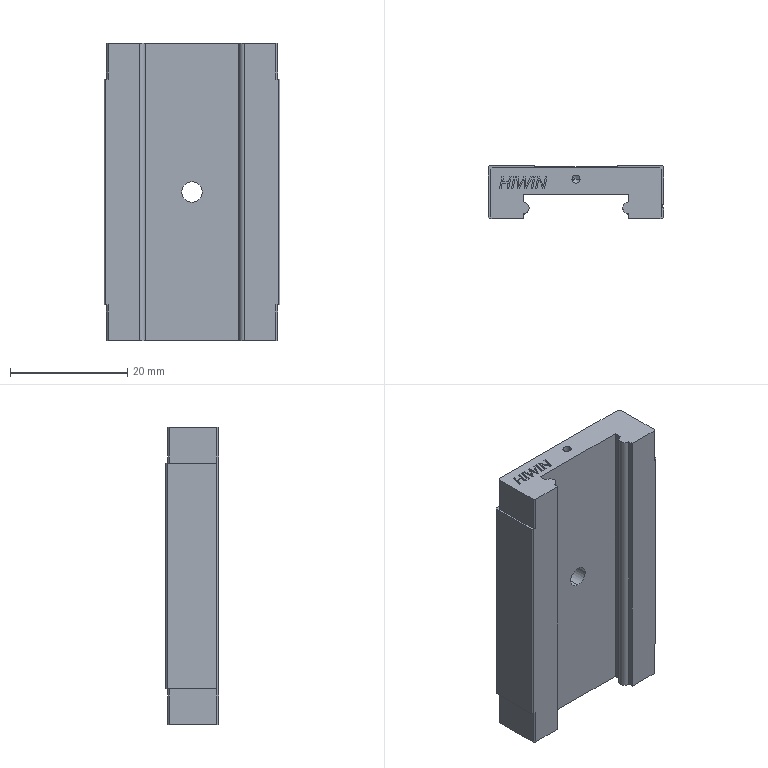Part | STEP file | Mount electronic clip MGW9H slider | 1 solid | 208 faces | box 30 x 9.1 x 50.7 mm | volume 9721 mm3 | plane 126 | spline 51 | cylinder 19 | cone 12 | commonest cylinder face diameters 3 x8 1.4 x4 2 x3 0.6 x2 3.5 x2